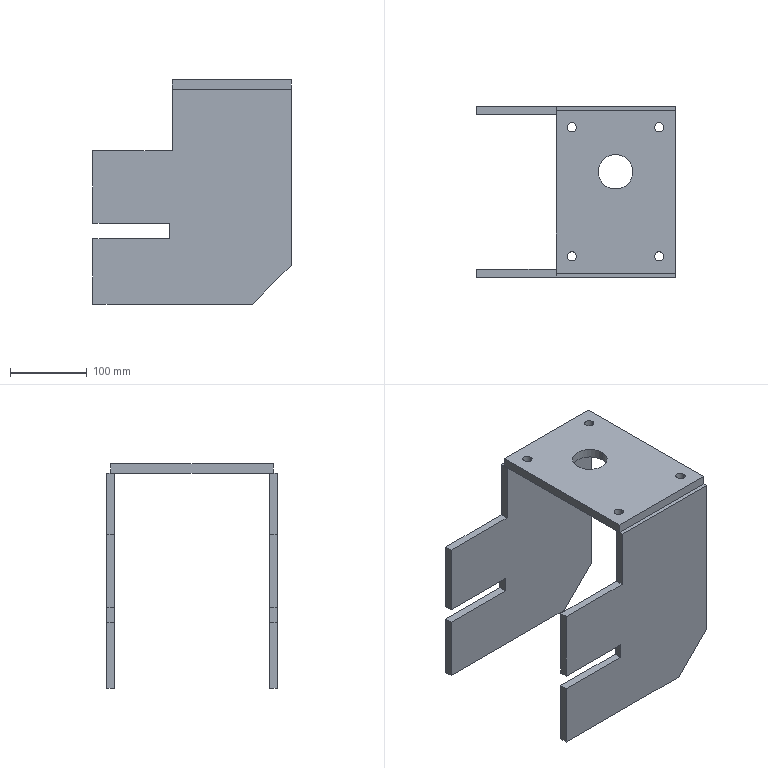Part | SolidWorks | features ICE 2, Chamfer 1, Cut 1, Extrusion 1, HoleWzd 1, MirrorSolid 1 | 3 solids | 42 faces | box 258 x 222 x 292 mm | volume 1584806 mm3 | plane 32 | cylinder 10 | commonest cylinder face diameters 12 x8 45 x2
STEP:
#1=CARTESIAN_POINT('',(22.5,26.,12.));
#2=VERTEX_POINT('',#1);
#3=CARTESIAN_POINT('',(-22.5,26.,12.));
#4=VERTEX_POINT('',#3);
#5=CARTESIAN_POINT('',(0.,26.,12.));
#6=DIRECTION('',(0.,0.,-1.));
#7=DIRECTION('',(1.,0.,0.));
#8=AXIS2_PLACEMENT_3D('',#5,#6,#7);
#9=CIRCLE('',#8,22.5);
#10=EDGE_CURVE('',#2,#4,#9,.T.);
#11=ORIENTED_EDGE('',*,*,#10,.F.);
#12=CARTESIAN_POINT('',(22.5,26.,0.));
#13=VERTEX_POINT('',#12);
#14=CARTESIAN_POINT('',(22.5,26.,12.001));
#15=DIRECTION('',(0.,0.,-1.));
#16=VECTOR('',#15,1000.);
#17=LINE('',#14,#16);
#18=EDGE_CURVE('',#2,#13,#17,.T.);
#19=ORIENTED_EDGE('',*,*,#18,.T.);
#20=CARTESIAN_POINT('',(-22.5,26.,0.));
#21=VERTEX_POINT('',#20);
#22=CARTESIAN_POINT('',(0.,26.,0.));
#23=DIRECTION('',(0.,0.,-1.));
#24=DIRECTION('',(-1.,0.,0.));
#25=AXIS2_PLACEMENT_3D('',#22,#23,#24);
#26=CIRCLE('',#25,22.5);
#27=EDGE_CURVE('',#13,#21,#26,.T.);
#28=ORIENTED_EDGE('',*,*,#27,.T.);
#29=CARTESIAN_POINT('',(-22.5,26.,12.001));
#30=DIRECTION('',(0.,0.,-1.));
#31=VECTOR('',#30,1000.);
#32=LINE('',#29,#31);
#33=EDGE_CURVE('',#4,#21,#32,.T.);
#34=ORIENTED_EDGE('',*,*,#33,.F.);
#35=EDGE_LOOP('',(#11,#19,#28,#34));
#36=FACE_OUTER_BOUND('',#35,.T.);
#37=CARTESIAN_POINT('',(0.,26.,12.001));
#38=DIRECTION('',(0.,0.,-1.));
#39=DIRECTION('',(-1.,0.,0.));
#40=AXIS2_PLACEMENT_3D('',#37,#38,#39);
#41=CYLINDRICAL_SURFACE('',#40,22.5);
#42=ADVANCED_FACE('',(#36),#41,.F.);
#43=CARTESIAN_POINT('',(51.,84.,12.));
#44=VERTEX_POINT('',#43);
#45=CARTESIAN_POINT('',(63.,84.,12.));
#46=VERTEX_POINT('',#45);
#47=CARTESIAN_POINT('',(57.,84.,12.));
#48=DIRECTION('',(0.,0.,1.));
#49=DIRECTION('',(1.,0.,0.));
#50=AXIS2_PLACEMENT_3D('',#47,#48,#49);
#51=CIRCLE('',#50,6.);
#52=EDGE_CURVE('',#44,#46,#51,.T.);
#53=ORIENTED_EDGE('',*,*,#52,.T.);
#54=CARTESIAN_POINT('',(63.,84.,0.));
#55=VERTEX_POINT('',#54);
#56=CARTESIAN_POINT('',(63.,84.,0.));
#57=DIRECTION('',(0.,0.,-1.));
#58=VECTOR('',#57,1000.);
#59=LINE('',#56,#58);
#60=EDGE_CURVE('',#46,#55,#59,.T.);
#61=ORIENTED_EDGE('',*,*,#60,.T.);
#62=CARTESIAN_POINT('',(51.,84.,0.));
#63=VERTEX_POINT('',#62);
#64=CARTESIAN_POINT('',(57.,84.,0.));
#65=DIRECTION('',(0.,0.,-1.));
#66=DIRECTION('',(-1.,0.,0.));
#67=AXIS2_PLACEMENT_3D('',#64,#65,#66);
#68=CIRCLE('',#67,6.);
#69=EDGE_CURVE('',#55,#63,#68,.T.);
#70=ORIENTED_EDGE('',*,*,#69,.T.);
#71=CARTESIAN_POINT('',(51.,84.,0.));
#72=DIRECTION('',(0.,0.,-1.));
#73=VECTOR('',#72,1000.);
#74=LINE('',#71,#73);
#75=EDGE_CURVE('',#44,#63,#74,.T.);
#76=ORIENTED_EDGE('',*,*,#75,.F.);
#77=EDGE_LOOP('',(#53,#61,#70,#76));
#78=FACE_OUTER_BOUND('',#77,.T.);
#79=CARTESIAN_POINT('',(57.,84.,0.));
#80=DIRECTION('',(0.,0.,-1.));
#81=DIRECTION('',(-1.,0.,0.));
#82=AXIS2_PLACEMENT_3D('',#79,#80,#81);
#83=CYLINDRICAL_SURFACE('',#82,6.);
#84=ADVANCED_FACE('',(#78),#83,.F.);
#85=CARTESIAN_POINT('',(-63.,84.,12.));
#86=VERTEX_POINT('',#85);
#87=CARTESIAN_POINT('',(-51.,84.,12.));
#88=VERTEX_POINT('',#87);
#89=CARTESIAN_POINT('',(-57.,84.,12.));
#90=DIRECTION('',(0.,0.,1.));
#91=DIRECTION('',(1.,0.,0.));
#92=AXIS2_PLACEMENT_3D('',#89,#90,#91);
#93=CIRCLE('',#92,6.);
#94=EDGE_CURVE('',#86,#88,#93,.T.);
#95=ORIENTED_EDGE('',*,*,#94,.T.);
#96=CARTESIAN_POINT('',(-51.,84.,0.));
#97=VERTEX_POINT('',#96);
#98=CARTESIAN_POINT('',(-51.,84.,0.));
#99=DIRECTION('',(0.,0.,-1.));
#100=VECTOR('',#99,1000.);
#101=LINE('',#98,#100);
#102=EDGE_CURVE('',#88,#97,#101,.T.);
#103=ORIENTED_EDGE('',*,*,#102,.T.);
#104=CARTESIAN_POINT('',(-63.,84.,0.));
#105=VERTEX_POINT('',#104);
#106=CARTESIAN_POINT('',(-57.,84.,0.));
#107=DIRECTION('',(0.,0.,-1.));
#108=DIRECTION('',(-1.,0.,0.));
#109=AXIS2_PLACEMENT_3D('',#106,#107,#108);
#110=CIRCLE('',#109,6.);
#111=EDGE_CURVE('',#97,#105,#110,.T.);
#112=ORIENTED_EDGE('',*,*,#111,.T.);
#113=CARTESIAN_POINT('',(-63.,84.,0.));
#114=DIRECTION('',(0.,0.,-1.));
#115=VECTOR('',#114,1000.);
#116=LINE('',#113,#115);
#117=EDGE_CURVE('',#86,#105,#116,.T.);
#118=ORIENTED_EDGE('',*,*,#117,.F.);
#119=EDGE_LOOP('',(#95,#103,#112,#118));
#120=FACE_OUTER_BOUND('',#119,.T.);
#121=CARTESIAN_POINT('',(-57.,84.,0.));
#122=DIRECTION('',(0.,0.,-1.));
#123=DIRECTION('',(-1.,0.,0.));
#124=AXIS2_PLACEMENT_3D('',#121,#122,#123);
#125=CYLINDRICAL_SURFACE('',#124,6.);
#126=ADVANCED_FACE('',(#120),#125,.F.);
#127=CARTESIAN_POINT('',(51.,-84.,12.));
#128=VERTEX_POINT('',#127);
#129=CARTESIAN_POINT('',(63.,-84.,12.));
#130=VERTEX_POINT('',#129);
#131=CARTESIAN_POINT('',(57.,-84.,12.));
#132=DIRECTION('',(0.,0.,1.));
#133=DIRECTION('',(1.,0.,0.));
#134=AXIS2_PLACEMENT_3D('',#131,#132,#133);
#135=CIRCLE('',#134,6.);
#136=EDGE_CURVE('',#128,#130,#135,.T.);
#137=ORIENTED_EDGE('',*,*,#136,.T.);
#138=CARTESIAN_POINT('',(63.,-84.,0.));
#139=VERTEX_POINT('',#138);
#140=CARTESIAN_POINT('',(63.,-84.,0.));
#141=DIRECTION('',(0.,0.,-1.));
#142=VECTOR('',#141,1000.);
#143=LINE('',#140,#142);
#144=EDGE_CURVE('',#130,#139,#143,.T.);
#145=ORIENTED_EDGE('',*,*,#144,.T.);
#146=CARTESIAN_POINT('',(51.,-84.,0.));
#147=VERTEX_POINT('',#146);
#148=CARTESIAN_POINT('',(57.,-84.,0.));
#149=DIRECTION('',(0.,0.,-1.));
#150=DIRECTION('',(-1.,0.,0.));
#151=AXIS2_PLACEMENT_3D('',#148,#149,#150);
#152=CIRCLE('',#151,6.);
#153=EDGE_CURVE('',#139,#147,#152,.T.);
#154=ORIENTED_EDGE('',*,*,#153,.T.);
#155=CARTESIAN_POINT('',(51.,-84.,0.));
#156=DIRECTION('',(0.,0.,-1.));
#157=VECTOR('',#156,1000.);
#158=LINE('',#155,#157);
#159=EDGE_CURVE('',#128,#147,#158,.T.);
#160=ORIENTED_EDGE('',*,*,#159,.F.);
#161=EDGE_LOOP('',(#137,#145,#154,#160));
#162=FACE_OUTER_BOUND('',#161,.T.);
#163=CARTESIAN_POINT('',(57.,-84.,0.));
#164=DIRECTION('',(0.,0.,-1.));
#165=DIRECTION('',(-1.,0.,0.));
#166=AXIS2_PLACEMENT_3D('',#163,#164,#165);
#167=CYLINDRICAL_SURFACE('',#166,6.);
#168=ADVANCED_FACE('',(#162),#167,.F.);
#169=CARTESIAN_POINT('',(-63.,-84.,12.));
#170=VERTEX_POINT('',#169);
#171=CARTESIAN_POINT('',(-51.,-84.,12.));
#172=VERTEX_POINT('',#171);
#173=CARTESIAN_POINT('',(-57.,-84.,12.));
#174=DIRECTION('',(0.,0.,1.));
#175=DIRECTION('',(1.,0.,0.));
#176=AXIS2_PLACEMENT_3D('',#173,#174,#175);
#177=CIRCLE('',#176,6.);
#178=EDGE_CURVE('',#170,#172,#177,.T.);
#179=ORIENTED_EDGE('',*,*,#178,.T.);
#180=CARTESIAN_POINT('',(-51.,-84.,0.));
#181=VERTEX_POINT('',#180);
#182=CARTESIAN_POINT('',(-51.,-84.,0.));
#183=DIRECTION('',(0.,0.,-1.));
#184=VECTOR('',#183,1000.);
#185=LINE('',#182,#184);
#186=EDGE_CURVE('',#172,#181,#185,.T.);
#187=ORIENTED_EDGE('',*,*,#186,.T.);
#188=CARTESIAN_POINT('',(-63.,-84.,0.));
#189=VERTEX_POINT('',#188);
#190=CARTESIAN_POINT('',(-57.,-84.,0.));
#191=DIRECTION('',(0.,0.,-1.));
#192=DIRECTION('',(-1.,0.,0.));
#193=AXIS2_PLACEMENT_3D('',#190,#191,#192);
#194=CIRCLE('',#193,6.);
#195=EDGE_CURVE('',#181,#189,#194,.T.);
#196=ORIENTED_EDGE('',*,*,#195,.T.);
#197=CARTESIAN_POINT('',(-63.,-84.,0.));
#198=DIRECTION('',(0.,0.,-1.));
#199=VECTOR('',#198,1000.);
#200=LINE('',#197,#199);
#201=EDGE_CURVE('',#170,#189,#200,.T.);
#202=ORIENTED_EDGE('',*,*,#201,.F.);
#203=EDGE_LOOP('',(#179,#187,#196,#202));
#204=FACE_OUTER_BOUND('',#203,.T.);
#205=CARTESIAN_POINT('',(-57.,-84.,0.));
#206=DIRECTION('',(0.,0.,-1.));
#207=DIRECTION('',(-1.,0.,0.));
#208=AXIS2_PLACEMENT_3D('',#205,#206,#207);
#209=CYLINDRICAL_SURFACE('',#208,6.);
#210=ADVANCED_FACE('',(#204),#209,.F.);
#211=CARTESIAN_POINT('',(0.,26.,0.));
#212=DIRECTION('',(0.,0.,-1.));
#213=DIRECTION('',(-1.,0.,0.));
#214=AXIS2_PLACEMENT_3D('',#211,#212,#213);
#215=CIRCLE('',#214,22.5);
#216=EDGE_CURVE('',#21,#13,#215,.T.);
#217=ORIENTED_EDGE('',*,*,#216,.F.);
#218=ORIENTED_EDGE('',*,*,#27,.F.);
#219=EDGE_LOOP('',(#217,#218));
#220=FACE_BOUND('',#219,.T.);
#221=CARTESIAN_POINT('',(57.,84.,0.));
#222=DIRECTION('',(0.,0.,-1.));
#223=DIRECTION('',(-1.,0.,0.));
#224=AXIS2_PLACEMENT_3D('',#221,#222,#223);
#225=CIRCLE('',#224,6.);
#226=EDGE_CURVE('',#63,#55,#225,.T.);
#227=ORIENTED_EDGE('',*,*,#226,.F.);
#228=ORIENTED_EDGE('',*,*,#69,.F.);
#229=EDGE_LOOP('',(#227,#228));
#230=FACE_BOUND('',#229,.T.);
#231=CARTESIAN_POINT('',(-57.,84.,0.));
#232=DIRECTION('',(0.,0.,-1.));
#233=DIRECTION('',(-1.,0.,0.));
#234=AXIS2_PLACEMENT_3D('',#231,#232,#233);
#235=CIRCLE('',#234,6.);
#236=EDGE_CURVE('',#105,#97,#235,.T.);
#237=ORIENTED_EDGE('',*,*,#236,.F.);
#238=ORIENTED_EDGE('',*,*,#111,.F.);
#239=EDGE_LOOP('',(#237,#238));
#240=FACE_BOUND('',#239,.T.);
#241=CARTESIAN_POINT('',(57.,-84.,0.));
#242=DIRECTION('',(0.,0.,-1.));
#243=DIRECTION('',(-1.,0.,0.));
#244=AXIS2_PLACEMENT_3D('',#241,#242,#243);
#245=CIRCLE('',#244,6.);
#246=EDGE_CURVE('',#147,#139,#245,.T.);
#247=ORIENTED_EDGE('',*,*,#246,.F.);
#248=ORIENTED_EDGE('',*,*,#153,.F.);
#249=EDGE_LOOP('',(#247,#248));
#250=FACE_BOUND('',#249,.T.);
#251=CARTESIAN_POINT('',(-77.5,106.,0.));
#252=VERTEX_POINT('',#251);
#253=CARTESIAN_POINT('',(-77.5,-106.,0.));
#254=VERTEX_POINT('',#253);
#255=CARTESIAN_POINT('',(-77.5,-106.,0.));
#256=DIRECTION('',(0.,-1.,0.));
#257=VECTOR('',#256,1000.);
#258=LINE('',#255,#257);
#259=EDGE_CURVE('',#252,#254,#258,.T.);
#260=ORIENTED_EDGE('',*,*,#259,.F.);
#261=CARTESIAN_POINT('',(77.5,106.,0.));
#262=VERTEX_POINT('',#261);
#263=CARTESIAN_POINT('',(77.5,106.,0.));
#264=DIRECTION('',(-1.,0.,0.));
#265=VECTOR('',#264,1000.);
#266=LINE('',#263,#265);
#267=EDGE_CURVE('',#262,#252,#266,.T.);
#268=ORIENTED_EDGE('',*,*,#267,.F.);
#269=CARTESIAN_POINT('',(77.5,-106.,0.));
#270=VERTEX_POINT('',#269);
#271=CARTESIAN_POINT('',(77.5,-106.,0.));
#272=DIRECTION('',(0.,1.,0.));
#273=VECTOR('',#272,1000.);
#274=LINE('',#271,#273);
#275=EDGE_CURVE('',#270,#262,#274,.T.);
#276=ORIENTED_EDGE('',*,*,#275,.F.);
#277=CARTESIAN_POINT('',(77.5,-106.,0.));
#278=DIRECTION('',(1.,0.,0.));
#279=VECTOR('',#278,1000.);
#280=LINE('',#277,#279);
#281=EDGE_CURVE('',#254,#270,#280,.T.);
#282=ORIENTED_EDGE('',*,*,#281,.F.);
#283=EDGE_LOOP('',(#260,#268,#276,#282));
#284=FACE_OUTER_BOUND('',#283,.T.);
#285=CARTESIAN_POINT('',(-57.,-84.,0.));
#286=DIRECTION('',(0.,0.,-1.));
#287=DIRECTION('',(-1.,0.,0.));
#288=AXIS2_PLACEMENT_3D('',#285,#286,#287);
#289=CIRCLE('',#288,6.);
#290=EDGE_CURVE('',#189,#181,#289,.T.);
#291=ORIENTED_EDGE('',*,*,#290,.F.);
#292=ORIENTED_EDGE('',*,*,#195,.F.);
#293=EDGE_LOOP('',(#291,#292));
#294=FACE_BOUND('',#293,.T.);
#295=CARTESIAN_POINT('',(0.,0.,0.));
#296=DIRECTION('',(0.,0.,1.));
#297=DIRECTION('',(1.,0.,0.));
#298=AXIS2_PLACEMENT_3D('',#295,#296,#297);
#299=PLANE('',#298);
#300=ADVANCED_FACE('',(#220,#230,#240,#250,#284,#294),#299,.F.);
#301=ORIENTED_EDGE('',*,*,#259,.T.);
#302=CARTESIAN_POINT('',(-77.5,-106.,12.));
#303=VERTEX_POINT('',#302);
#304=CARTESIAN_POINT('',(-77.5,-106.,12.));
#305=DIRECTION('',(0.,0.,-1.));
#306=VECTOR('',#305,1000.);
#307=LINE('',#304,#306);
#308=EDGE_CURVE('',#303,#254,#307,.T.);
#309=ORIENTED_EDGE('',*,*,#308,.F.);
#310=CARTESIAN_POINT('',(-77.5,106.,12.));
#311=VERTEX_POINT('',#310);
#312=CARTESIAN_POINT('',(-77.5,-106.,12.));
#313=DIRECTION('',(0.,-1.,0.));
#314=VECTOR('',#313,1000.);
#315=LINE('',#312,#314);
#316=EDGE_CURVE('',#311,#303,#315,.T.);
#317=ORIENTED_EDGE('',*,*,#316,.F.);
#318=CARTESIAN_POINT('',(-77.5,106.,12.));
#319=DIRECTION('',(0.,0.,-1.));
#320=VECTOR('',#319,1000.);
#321=LINE('',#318,#320);
#322=EDGE_CURVE('',#311,#252,#321,.T.);
#323=ORIENTED_EDGE('',*,*,#322,.T.);
#324=EDGE_LOOP('',(#301,#309,#317,#323));
#325=FACE_OUTER_BOUND('',#324,.T.);
#326=CARTESIAN_POINT('',(-77.5,-106.,12.));
#327=DIRECTION('',(1.,0.,0.));
#328=DIRECTION('',(0.,0.,-1.));
#329=AXIS2_PLACEMENT_3D('',#326,#327,#328);
#330=PLANE('',#329);
#331=ADVANCED_FACE('',(#325),#330,.F.);
#332=ORIENTED_EDGE('',*,*,#281,.T.);
#333=CARTESIAN_POINT('',(77.5,-106.,12.));
#334=VERTEX_POINT('',#333);
#335=CARTESIAN_POINT('',(77.5,-106.,12.));
#336=DIRECTION('',(0.,0.,-1.));
#337=VECTOR('',#336,1000.);
#338=LINE('',#335,#337);
#339=EDGE_CURVE('',#334,#270,#338,.T.);
#340=ORIENTED_EDGE('',*,*,#339,.F.);
#341=CARTESIAN_POINT('',(77.5,-106.,12.));
#342=DIRECTION('',(1.,0.,0.));
#343=VECTOR('',#342,1000.);
#344=LINE('',#341,#343);
#345=EDGE_CURVE('',#303,#334,#344,.T.);
#346=ORIENTED_EDGE('',*,*,#345,.F.);
#347=ORIENTED_EDGE('',*,*,#308,.T.);
#348=EDGE_LOOP('',(#332,#340,#346,#347));
#349=FACE_OUTER_BOUND('',#348,.T.);
#350=CARTESIAN_POINT('',(77.5,-106.,12.));
#351=DIRECTION('',(0.,1.,0.));
#352=DIRECTION('',(0.,0.,1.));
#353=AXIS2_PLACEMENT_3D('',#350,#351,#352);
#354=PLANE('',#353);
#355=ADVANCED_FACE('',(#349),#354,.F.);
#356=ORIENTED_EDGE('',*,*,#275,.T.);
#357=CARTESIAN_POINT('',(77.5,106.,12.));
#358=VERTEX_POINT('',#357);
#359=CARTESIAN_POINT('',(77.5,106.,12.));
#360=DIRECTION('',(0.,0.,-1.));
#361=VECTOR('',#360,1000.);
#362=LINE('',#359,#361);
#363=EDGE_CURVE('',#358,#262,#362,.T.);
#364=ORIENTED_EDGE('',*,*,#363,.F.);
#365=CARTESIAN_POINT('',(77.5,-106.,12.));
#366=DIRECTION('',(0.,1.,0.));
#367=VECTOR('',#366,1000.);
#368=LINE('',#365,#367);
#369=EDGE_CURVE('',#334,#358,#368,.T.);
#370=ORIENTED_EDGE('',*,*,#369,.F.);
#371=ORIENTED_EDGE('',*,*,#339,.T.);
#372=EDGE_LOOP('',(#356,#364,#370,#371));
#373=FACE_OUTER_BOUND('',#372,.T.);
#374=CARTESIAN_POINT('',(77.5,-106.,12.));
#375=DIRECTION('',(-1.,0.,0.));
#376=DIRECTION('',(0.,0.,1.));
#377=AXIS2_PLACEMENT_3D('',#374,#375,#376);
#378=PLANE('',#377);
#379=ADVANCED_FACE('',(#373),#378,.F.);
#380=ORIENTED_EDGE('',*,*,#267,.T.);
#381=ORIENTED_EDGE('',*,*,#322,.F.);
#382=CARTESIAN_POINT('',(77.5,106.,12.));
#383=DIRECTION('',(-1.,0.,0.));
#384=VECTOR('',#383,1000.);
#385=LINE('',#382,#384);
#386=EDGE_CURVE('',#358,#311,#385,.T.);
#387=ORIENTED_EDGE('',*,*,#386,.F.);
#388=ORIENTED_EDGE('',*,*,#363,.T.);
#389=EDGE_LOOP('',(#380,#381,#387,#388));
#390=FACE_OUTER_BOUND('',#389,.T.);
#391=CARTESIAN_POINT('',(77.5,106.,12.));
#392=DIRECTION('',(0.,-1.,0.));
#393=DIRECTION('',(0.,0.,-1.));
#394=AXIS2_PLACEMENT_3D('',#391,#392,#393);
#395=PLANE('',#394);
#396=ADVANCED_FACE('',(#390),#395,.F.);
#397=CARTESIAN_POINT('',(0.,26.,12.));
#398=DIRECTION('',(0.,0.,-1.));
#399=DIRECTION('',(1.,0.,0.));
#400=AXIS2_PLACEMENT_3D('',#397,#398,#399);
#401=CIRCLE('',#400,22.5);
#402=EDGE_CURVE('',#4,#2,#401,.T.);
#403=ORIENTED_EDGE('',*,*,#402,.T.);
#404=ORIENTED_EDGE('',*,*,#10,.T.);
#405=EDGE_LOOP('',(#403,#404));
#406=FACE_BOUND('',#405,.T.);
#407=ORIENTED_EDGE('',*,*,#52,.F.);
#408=CARTESIAN_POINT('',(57.,84.,12.));
#409=DIRECTION('',(0.,0.,1.));
#410=DIRECTION('',(1.,0.,0.));
#411=AXIS2_PLACEMENT_3D('',#408,#409,#410);
#412=CIRCLE('',#411,6.);
#413=EDGE_CURVE('',#46,#44,#412,.T.);
#414=ORIENTED_EDGE('',*,*,#413,.F.);
#415=EDGE_LOOP('',(#407,#414));
#416=FACE_BOUND('',#415,.T.);
#417=ORIENTED_EDGE('',*,*,#94,.F.);
#418=CARTESIAN_POINT('',(-57.,84.,12.));
#419=DIRECTION('',(0.,0.,1.));
#420=DIRECTION('',(1.,0.,0.));
#421=AXIS2_PLACEMENT_3D('',#418,#419,#420);
#422=CIRCLE('',#421,6.);
#423=EDGE_CURVE('',#88,#86,#422,.T.);
#424=ORIENTED_EDGE('',*,*,#423,.F.);
#425=EDGE_LOOP('',(#417,#424));
#426=FACE_BOUND('',#425,.T.);
#427=ORIENTED_EDGE('',*,*,#136,.F.);
#428=CARTESIAN_POINT('',(57.,-84.,12.));
#429=DIRECTION('',(0.,0.,1.));
#430=DIRECTION('',(1.,0.,0.));
#431=AXIS2_PLACEMENT_3D('',#428,#429,#430);
#432=CIRCLE('',#431,6.);
#433=EDGE_CURVE('',#130,#128,#432,.T.);
#434=ORIENTED_EDGE('',*,*,#433,.F.);
#435=EDGE_LOOP('',(#427,#434));
#436=FACE_BOUND('',#435,.T.);
#437=ORIENTED_EDGE('',*,*,#178,.F.);
#438=CARTESIAN_POINT('',(-57.,-84.,12.));
#439=DIRECTION('',(0.,0.,1.));
#440=DIRECTION('',(1.,0.,0.));
#441=AXIS2_PLACEMENT_3D('',#438,#439,#440);
#442=CIRCLE('',#441,6.);
#443=EDGE_CURVE('',#172,#170,#442,.T.);
#444=ORIENTED_EDGE('',*,*,#443,.F.);
#445=EDGE_LOOP('',(#437,#444));
#446=FACE_BOUND('',#445,.T.);
#447=ORIENTED_EDGE('',*,*,#316,.T.);
#448=ORIENTED_EDGE('',*,*,#345,.T.);
#449=ORIENTED_EDGE('',*,*,#369,.T.);
#450=ORIENTED_EDGE('',*,*,#386,.T.);
#451=EDGE_LOOP('',(#447,#448,#449,#450));
#452=FACE_OUTER_BOUND('',#451,.T.);
#453=CARTESIAN_POINT('',(0.,0.,12.));
#454=DIRECTION('',(0.,0.,1.));
#455=DIRECTION('',(1.,0.,0.));
#456=AXIS2_PLACEMENT_3D('',#453,#454,#455);
#457=PLANE('',#456);
#458=ADVANCED_FACE('',(#406,#416,#426,#436,#446,#452),#457,.T.);
#459=ORIENTED_EDGE('',*,*,#186,.F.);
#460=ORIENTED_EDGE('',*,*,#443,.T.);
#461=ORIENTED_EDGE('',*,*,#201,.T.);
#462=ORIENTED_EDGE('',*,*,#290,.T.);
#463=EDGE_LOOP('',(#459,#460,#461,#462));
#464=FACE_OUTER_BOUND('',#463,.T.);
#465=CARTESIAN_POINT('',(-57.,-84.,0.));
#466=DIRECTION('',(0.,0.,-1.));
#467=DIRECTION('',(-1.,0.,0.));
#468=AXIS2_PLACEMENT_3D('',#465,#466,#467);
#469=CYLINDRICAL_SURFACE('',#468,6.);
#470=ADVANCED_FACE('',(#464),#469,.F.);
#471=ORIENTED_EDGE('',*,*,#144,.F.);
#472=ORIENTED_EDGE('',*,*,#433,.T.);
#473=ORIENTED_EDGE('',*,*,#159,.T.);
#474=ORIENTED_EDGE('',*,*,#246,.T.);
#475=EDGE_LOOP('',(#471,#472,#473,#474));
#476=FACE_OUTER_BOUND('',#475,.T.);
#477=CARTESIAN_POINT('',(57.,-84.,0.));
#478=DIRECTION('',(0.,0.,-1.));
#479=DIRECTION('',(-1.,0.,0.));
#480=AXIS2_PLACEMENT_3D('',#477,#478,#479);
#481=CYLINDRICAL_SURFACE('',#480,6.);
#482=ADVANCED_FACE('',(#476),#481,.F.);
#483=ORIENTED_EDGE('',*,*,#102,.F.);
#484=ORIENTED_EDGE('',*,*,#423,.T.);
#485=ORIENTED_EDGE('',*,*,#117,.T.);
#486=ORIENTED_EDGE('',*,*,#236,.T.);
#487=EDGE_LOOP('',(#483,#484,#485,#486));
#488=FACE_OUTER_BOUND('',#487,.T.);
#489=CARTESIAN_POINT('',(-57.,84.,0.));
#490=DIRECTION('',(0.,0.,-1.));
#491=DIRECTION('',(-1.,0.,0.));
#492=AXIS2_PLACEMENT_3D('',#489,#490,#491);
#493=CYLINDRICAL_SURFACE('',#492,6.);
#494=ADVANCED_FACE('',(#488),#493,.F.);
#495=ORIENTED_EDGE('',*,*,#60,.F.);
#496=ORIENTED_EDGE('',*,*,#413,.T.);
#497=ORIENTED_EDGE('',*,*,#75,.T.);
#498=ORIENTED_EDGE('',*,*,#226,.T.);
#499=EDGE_LOOP('',(#495,#496,#497,#498));
#500=FACE_OUTER_BOUND('',#499,.T.);
#501=CARTESIAN_POINT('',(57.,84.,0.));
#502=DIRECTION('',(0.,0.,-1.));
#503=DIRECTION('',(-1.,0.,0.));
#504=AXIS2_PLACEMENT_3D('',#501,#502,#503);
#505=CYLINDRICAL_SURFACE('',#504,6.);
#506=ADVANCED_FACE('',(#500),#505,.F.);
#507=ORIENTED_EDGE('',*,*,#18,.F.);
#508=ORIENTED_EDGE('',*,*,#402,.F.);
#509=ORIENTED_EDGE('',*,*,#33,.T.);
#510=ORIENTED_EDGE('',*,*,#216,.T.);
#511=EDGE_LOOP('',(#507,#508,#509,#510));
#512=FACE_OUTER_BOUND('',#511,.T.);
#513=CARTESIAN_POINT('',(0.,26.,12.001));
#514=DIRECTION('',(0.,0.,-1.));
#515=DIRECTION('',(-1.,0.,0.));
#516=AXIS2_PLACEMENT_3D('',#513,#514,#515);
#517=CYLINDRICAL_SURFACE('',#516,22.5);
#518=ADVANCED_FACE('',(#512),#517,.F.);
#519=CLOSED_SHELL('',(#42,#84,#126,#168,#210,#300,#331,#355,#379,#396,#458,#470,#482,#494,#506,#518));
#520=MANIFOLD_SOLID_BREP('',#519);
#521=CARTESIAN_POINT('',(-180.5,101.,-280.));
#522=VERTEX_POINT('',#521);
#523=CARTESIAN_POINT('',(-180.5,101.,-195.));
#524=VERTEX_POINT('',#523);
#525=CARTESIAN_POINT('',(-180.5,101.,-280.));
#526=DIRECTION('',(0.,0.,1.));
#527=VECTOR('',#526,1000.);
#528=LINE('',#525,#527);
#529=EDGE_CURVE('',#522,#524,#528,.T.);
#530=ORIENTED_EDGE('',*,*,#529,.T.);
#531=CARTESIAN_POINT('',(-180.5,111.,-195.));
#532=VERTEX_POINT('',#531);
#533=CARTESIAN_POINT('',(-180.5,-111.,-195.));
#534=DIRECTION('',(0.,1.,0.));
#535=VECTOR('',#534,1000.);
#536=LINE('',#533,#535);
#537=EDGE_CURVE('',#524,#532,#536,.T.);
#538=ORIENTED_EDGE('',*,*,#537,.T.);
#539=CARTESIAN_POINT('',(-180.5,111.,-280.));
#540=VERTEX_POINT('',#539);
#541=CARTESIAN_POINT('',(-180.5,111.,-280.));
#542=DIRECTION('',(0.,0.,1.));
#543=VECTOR('',#542,1000.);
#544=LINE('',#541,#543);
#545=EDGE_CURVE('',#540,#532,#544,.T.);
#546=ORIENTED_EDGE('',*,*,#545,.F.);
#547=CARTESIAN_POINT('',(-180.5,111.,-280.));
#548=DIRECTION('',(0.,-1.,0.));
#549=VECTOR('',#548,1000.);
#550=LINE('',#547,#549);
#551=EDGE_CURVE('',#540,#522,#550,.T.);
#552=ORIENTED_EDGE('',*,*,#551,.T.);
#553=EDGE_LOOP('',(#530,#538,#546,#552));
#554=FACE_OUTER_BOUND('',#553,.T.);
#555=CARTESIAN_POINT('',(-180.5,111.,-280.));
#556=DIRECTION('',(1.,0.,0.));
#557=DIRECTION('',(0.,0.,-1.));
#558=AXIS2_PLACEMENT_3D('',#555,#556,#557);
#559=PLANE('',#558);
#560=ADVANCED_FACE('',(#554),#559,.F.);
#561=CARTESIAN_POINT('',(77.5,101.,0.));
#562=VERTEX_POINT('',#561);
#563=CARTESIAN_POINT('',(77.5,101.,-230.));
#564=VERTEX_POINT('',#563);
#565=CARTESIAN_POINT('',(77.5,101.,0.));
#566=DIRECTION('',(0.,0.,-1.));
#567=VECTOR('',#566,1000.);
#568=LINE('',#565,#567);
#569=EDGE_CURVE('',#562,#564,#568,.T.);
#570=ORIENTED_EDGE('',*,*,#569,.T.);
#571=CARTESIAN_POINT('',(77.5,111.,-230.));
#572=VERTEX_POINT('',#571);
#573=CARTESIAN_POINT('',(77.5,111.,-230.));
#574=DIRECTION('',(0.,1.,0.));
#575=VECTOR('',#574,1000.);
#576=LINE('',#573,#575);
#577=EDGE_CURVE('',#564,#572,#576,.T.);
#578=ORIENTED_EDGE('',*,*,#577,.T.);
#579=CARTESIAN_POINT('',(77.5,111.,0.));
#580=VERTEX_POINT('',#579);
#581=CARTESIAN_POINT('',(77.5,111.,0.));
#582=DIRECTION('',(0.,0.,-1.));
#583=VECTOR('',#582,1000.);
#584=LINE('',#581,#583);
#585=EDGE_CURVE('',#580,#572,#584,.T.);
#586=ORIENTED_EDGE('',*,*,#585,.F.);
#587=CARTESIAN_POINT('',(77.5,111.,0.));
#588=DIRECTION('',(0.,-1.,0.));
#589=VECTOR('',#588,1000.);
#590=LINE('',#587,#589);
#591=EDGE_CURVE('',#580,#562,#590,.T.);
#592=ORIENTED_EDGE('',*,*,#591,.T.);
#593=EDGE_LOOP('',(#570,#578,#586,#592));
#594=FACE_OUTER_BOUND('',#593,.T.);
#595=CARTESIAN_POINT('',(77.5,111.,0.));
#596=DIRECTION('',(-1.,0.,0.));
#597=DIRECTION('',(0.,0.,1.));
#598=AXIS2_PLACEMENT_3D('',#595,#596,#597);
#599=PLANE('',#598);
#600=ADVANCED_FACE('',(#594),#599,.F.);
#601=CARTESIAN_POINT('',(27.5,111.,-280.));
#602=VERTEX_POINT('',#601);
#603=CARTESIAN_POINT('',(77.5,111.,-280.));
#604=DIRECTION('',(-1.,0.,0.));
#605=VECTOR('',#604,1000.);
#606=LINE('',#603,#605);
#607=EDGE_CURVE('',#602,#540,#606,.T.);
#608=ORIENTED_EDGE('',*,*,#607,.F.);
#609=CARTESIAN_POINT('',(27.5,101.,-280.));
#610=VERTEX_POINT('',#609);
#611=CARTESIAN_POINT('',(27.5,111.,-280.));
#612=DIRECTION('',(0.,-1.,0.));
#613=VECTOR('',#612,1000.);
#614=LINE('',#611,#613);
#615=EDGE_CURVE('',#602,#610,#614,.T.);
#616=ORIENTED_EDGE('',*,*,#615,.T.);
#617=CARTESIAN_POINT('',(77.5,101.,-280.));
#618=DIRECTION('',(-1.,0.,0.));
#619=VECTOR('',#618,1000.);
#620=LINE('',#617,#619);
#621=EDGE_CURVE('',#610,#522,#620,.T.);
#622=ORIENTED_EDGE('',*,*,#621,.T.);
#623=ORIENTED_EDGE('',*,*,#551,.F.);
#624=EDGE_LOOP('',(#608,#616,#622,#623));
#625=FACE_OUTER_BOUND('',#624,.T.);
#626=CARTESIAN_POINT('',(77.5,111.,-280.));
#627=DIRECTION('',(0.,0.,1.));
#628=DIRECTION('',(1.,0.,0.));
#629=AXIS2_PLACEMENT_3D('',#626,#627,#628);
#630=PLANE('',#629);
#631=ADVANCED_FACE('',(#625),#630,.F.);
#632=CARTESIAN_POINT('',(-180.5,111.,-175.));
#633=VERTEX_POINT('',#632);
#634=CARTESIAN_POINT('',(-180.5,111.,-80.));
#635=VERTEX_POINT('',#634);
#636=CARTESIAN_POINT('',(-180.5,111.,-280.));
#637=DIRECTION('',(0.,0.,1.));
#638=VECTOR('',#637,1000.);
#639=LINE('',#636,#638);
#640=EDGE_CURVE('',#633,#635,#639,.T.);
#641=ORIENTED_EDGE('',*,*,#640,.F.);
#642=CARTESIAN_POINT('',(-180.5,101.,-175.));
#643=VERTEX_POINT('',#642);
#644=CARTESIAN_POINT('',(-180.5,-111.,-175.));
#645=DIRECTION('',(0.,1.,0.));
#646=VECTOR('',#645,1000.);
#647=LINE('',#644,#646);
#648=EDGE_CURVE('',#643,#633,#647,.T.);
#649=ORIENTED_EDGE('',*,*,#648,.F.);
#650=CARTESIAN_POINT('',(-180.5,101.,-80.));
#651=VERTEX_POINT('',#650);
#652=CARTESIAN_POINT('',(-180.5,101.,-280.));
#653=DIRECTION('',(0.,0.,1.));
#654=VECTOR('',#653,1000.);
#655=LINE('',#652,#654);
#656=EDGE_CURVE('',#643,#651,#655,.T.);
#657=ORIENTED_EDGE('',*,*,#656,.T.);
#658=CARTESIAN_POINT('',(-180.5,111.,-80.));
#659=DIRECTION('',(0.,-1.,0.));
#660=VECTOR('',#659,1000.);
#661=LINE('',#658,#660);
#662=EDGE_CURVE('',#635,#651,#661,.T.);
#663=ORIENTED_EDGE('',*,*,#662,.F.);
#664=EDGE_LOOP('',(#641,#649,#657,#663));
#665=FACE_OUTER_BOUND('',#664,.T.);
#666=CARTESIAN_POINT('',(-180.5,111.,-280.));
#667=DIRECTION('',(1.,0.,0.));
#668=DIRECTION('',(0.,0.,-1.));
#669=AXIS2_PLACEMENT_3D('',#666,#667,#668);
#670=PLANE('',#669);
#671=ADVANCED_FACE('',(#665),#670,.F.);
#672=CARTESIAN_POINT('',(-77.5,101.,-80.));
#673=VERTEX_POINT('',#672);
#674=CARTESIAN_POINT('',(-77.5,101.,-80.));
#675=DIRECTION('',(1.,0.,0.));
#676=VECTOR('',#675,1000.);
#677=LINE('',#674,#676);
#678=EDGE_CURVE('',#651,#673,#677,.T.);
#679=ORIENTED_EDGE('',*,*,#678,.T.);
#680=CARTESIAN_POINT('',(-77.5,111.,-80.));
#681=VERTEX_POINT('',#680);
#682=CARTESIAN_POINT('',(-77.5,111.,-80.));
#683=DIRECTION('',(0.,-1.,0.));
#684=VECTOR('',#683,1000.);
#685=LINE('',#682,#684);
#686=EDGE_CURVE('',#681,#673,#685,.T.);
#687=ORIENTED_EDGE('',*,*,#686,.F.);
#688=CARTESIAN_POINT('',(-77.5,111.,-80.));
#689=DIRECTION('',(1.,0.,0.));
#690=VECTOR('',#689,1000.);
#691=LINE('',#688,#690);
#692=EDGE_CURVE('',#635,#681,#691,.T.);
#693=ORIENTED_EDGE('',*,*,#692,.F.);
#694=ORIENTED_EDGE('',*,*,#662,.T.);
#695=EDGE_LOOP('',(#679,#687,#693,#694));
#696=FACE_OUTER_BOUND('',#695,.T.);
#697=CARTESIAN_POINT('',(-77.5,111.,-80.));
#698=DIRECTION('',(0.,0.,-1.));
#699=DIRECTION('',(-1.,0.,0.));
#700=AXIS2_PLACEMENT_3D('',#697,#698,#699);
#701=PLANE('',#700);
#702=ADVANCED_FACE('',(#696),#701,.F.);
#703=CARTESIAN_POINT('',(-77.5,101.,0.));
#704=VERTEX_POINT('',#703);
#705=CARTESIAN_POINT('',(-77.5,101.,0.));
#706=DIRECTION('',(0.,0.,1.));
#707=VECTOR('',#706,1000.);
#708=LINE('',#705,#707);
#709=EDGE_CURVE('',#673,#704,#708,.T.);
#710=ORIENTED_EDGE('',*,*,#709,.T.);
#711=CARTESIAN_POINT('',(-77.5,111.,0.));
#712=VERTEX_POINT('',#711);
#713=CARTESIAN_POINT('',(-77.5,111.,0.));
#714=DIRECTION('',(0.,-1.,0.));
#715=VECTOR('',#714,1000.);
#716=LINE('',#713,#715);
#717=EDGE_CURVE('',#712,#704,#716,.T.);
#718=ORIENTED_EDGE('',*,*,#717,.F.);
#719=CARTESIAN_POINT('',(-77.5,111.,0.));
#720=DIRECTION('',(0.,0.,1.));
#721=VECTOR('',#720,1000.);
#722=LINE('',#719,#721);
#723=EDGE_CURVE('',#681,#712,#722,.T.);
#724=ORIENTED_EDGE('',*,*,#723,.F.);
#725=ORIENTED_EDGE('',*,*,#686,.T.);
#726=EDGE_LOOP('',(#710,#718,#724,#725));
#727=FACE_OUTER_BOUND('',#726,.T.);
#728=CARTESIAN_POINT('',(-77.5,111.,0.));
#729=DIRECTION('',(1.,0.,0.));
#730=DIRECTION('',(0.,0.,-1.));
#731=AXIS2_PLACEMENT_3D('',#728,#729,#730);
#732=PLANE('',#731);
#733=ADVANCED_FACE('',(#727),#732,.F.);
#734=CARTESIAN_POINT('',(77.5,101.,0.));
#735=DIRECTION('',(1.,0.,0.));
#736=VECTOR('',#735,1000.);
#737=LINE('',#734,#736);
#738=EDGE_CURVE('',#704,#562,#737,.T.);
#739=ORIENTED_EDGE('',*,*,#738,.T.);
#740=ORIENTED_EDGE('',*,*,#591,.F.);
#741=CARTESIAN_POINT('',(77.5,111.,0.));
#742=DIRECTION('',(1.,0.,0.));
#743=VECTOR('',#742,1000.);
#744=LINE('',#741,#743);
#745=EDGE_CURVE('',#712,#580,#744,.T.);
#746=ORIENTED_EDGE('',*,*,#745,.F.);
#747=ORIENTED_EDGE('',*,*,#717,.T.);
#748=EDGE_LOOP('',(#739,#740,#746,#747));
#749=FACE_OUTER_BOUND('',#748,.T.);
#750=CARTESIAN_POINT('',(77.5,111.,0.));
#751=DIRECTION('',(0.,0.,-1.));
#752=DIRECTION('',(-1.,0.,0.));
#753=AXIS2_PLACEMENT_3D('',#750,#751,#752);
#754=PLANE('',#753);
#755=ADVANCED_FACE('',(#749),#754,.F.);
#756=CARTESIAN_POINT('',(-80.5,111.,-195.));
#757=VERTEX_POINT('',#756);
#758=CARTESIAN_POINT('',(-180.5,111.,-195.));
#759=DIRECTION('',(-1.,0.,0.));
#760=VECTOR('',#759,1000.);
#761=LINE('',#758,#760);
#762=EDGE_CURVE('',#757,#532,#761,.T.);
#763=ORIENTED_EDGE('',*,*,#762,.F.);
#764=CARTESIAN_POINT('',(-80.5,111.,-175.));
#765=VERTEX_POINT('',#764);
#766=CARTESIAN_POINT('',(-80.5,111.,-195.));
#767=DIRECTION('',(0.,0.,-1.));
#768=VECTOR('',#767,1000.);
#769=LINE('',#766,#768);
#770=EDGE_CURVE('',#765,#757,#769,.T.);
#771=ORIENTED_EDGE('',*,*,#770,.F.);
#772=CARTESIAN_POINT('',(-180.5,111.,-175.));
#773=DIRECTION('',(1.,0.,0.));
#774=VECTOR('',#773,1000.);
#775=LINE('',#772,#774);
#776=EDGE_CURVE('',#633,#765,#775,.T.);
#777=ORIENTED_EDGE('',*,*,#776,.F.);
#778=ORIENTED_EDGE('',*,*,#640,.T.);
#779=ORIENTED_EDGE('',*,*,#692,.T.);
#780=ORIENTED_EDGE('',*,*,#723,.T.);
#781=ORIENTED_EDGE('',*,*,#745,.T.);
#782=ORIENTED_EDGE('',*,*,#585,.T.);
#783=CARTESIAN_POINT('',(153.75,111.,-153.75));
#784=DIRECTION('',(-0.7071,0.,-0.7071));
#785=VECTOR('',#784,1000.);
#786=LINE('',#783,#785);
#787=EDGE_CURVE('',#572,#602,#786,.T.);
#788=ORIENTED_EDGE('',*,*,#787,.T.);
#789=ORIENTED_EDGE('',*,*,#607,.T.);
#790=ORIENTED_EDGE('',*,*,#545,.T.);
#791=EDGE_LOOP('',(#763,#771,#777,#778,#779,#780,#781,#782,#788,#789,#790));
#792=FACE_OUTER_BOUND('',#791,.T.);
#793=CARTESIAN_POINT('',(0.,111.,0.));
#794=DIRECTION('',(0.,1.,0.));
#795=DIRECTION('',(0.,0.,1.));
#796=AXIS2_PLACEMENT_3D('',#793,#794,#795);
#797=PLANE('',#796);
#798=ADVANCED_FACE('',(#792),#797,.T.);
#799=CARTESIAN_POINT('',(-80.5,101.,-175.));
#800=VERTEX_POINT('',#799);
#801=CARTESIAN_POINT('',(-80.5,101.,-195.));
#802=VERTEX_POINT('',#801);
#803=CARTESIAN_POINT('',(-80.5,101.,0.));
#804=DIRECTION('',(0.,0.,-1.));
#805=VECTOR('',#804,1000.);
#806=LINE('',#803,#805);
#807=EDGE_CURVE('',#800,#802,#806,.T.);
#808=ORIENTED_EDGE('',*,*,#807,.T.);
#809=CARTESIAN_POINT('',(0.,101.,-195.));
#810=DIRECTION('',(-1.,0.,0.));
#811=VECTOR('',#810,1000.);
#812=LINE('',#809,#811);
#813=EDGE_CURVE('',#802,#524,#812,.T.);
#814=ORIENTED_EDGE('',*,*,#813,.T.);
#815=ORIENTED_EDGE('',*,*,#529,.F.);
#816=ORIENTED_EDGE('',*,*,#621,.F.);
#817=CARTESIAN_POINT('',(27.5,101.,-280.));
#818=DIRECTION('',(0.7071,0.,0.7071));
#819=VECTOR('',#818,1000.);
#820=LINE('',#817,#819);
#821=EDGE_CURVE('',#610,#564,#820,.T.);
#822=ORIENTED_EDGE('',*,*,#821,.T.);
#823=ORIENTED_EDGE('',*,*,#569,.F.);
#824=ORIENTED_EDGE('',*,*,#738,.F.);
#825=ORIENTED_EDGE('',*,*,#709,.F.);
#826=ORIENTED_EDGE('',*,*,#678,.F.);
#827=ORIENTED_EDGE('',*,*,#656,.F.);
#828=CARTESIAN_POINT('',(0.,101.,-175.));
#829=DIRECTION('',(1.,0.,0.));
#830=VECTOR('',#829,1000.);
#831=LINE('',#828,#830);
#832=EDGE_CURVE('',#643,#800,#831,.T.);
#833=ORIENTED_EDGE('',*,*,#832,.T.);
#834=EDGE_LOOP('',(#808,#814,#815,#816,#822,#823,#824,#825,#826,#827,#833));
#835=FACE_OUTER_BOUND('',#834,.T.);
#836=CARTESIAN_POINT('',(0.,101.,0.));
#837=DIRECTION('',(0.,1.,0.));
#838=DIRECTION('',(0.,0.,1.));
#839=AXIS2_PLACEMENT_3D('',#836,#837,#838);
#840=PLANE('',#839);
#841=ADVANCED_FACE('',(#835),#840,.F.);
#842=ORIENTED_EDGE('',*,*,#787,.F.);
#843=ORIENTED_EDGE('',*,*,#577,.F.);
#844=ORIENTED_EDGE('',*,*,#821,.F.);
#845=ORIENTED_EDGE('',*,*,#615,.F.);
#846=EDGE_LOOP('',(#842,#843,#844,#845));
#847=FACE_OUTER_BOUND('',#846,.T.);
#848=CARTESIAN_POINT('',(27.5,111.,-280.));
#849=DIRECTION('',(-0.7071,0.,0.7071));
#850=DIRECTION('',(0.,-1.,0.));
#851=AXIS2_PLACEMENT_3D('',#848,#849,#850);
#852=PLANE('',#851);
#853=ADVANCED_FACE('',(#847),#852,.F.);
#854=CARTESIAN_POINT('',(-80.5,-111.,-195.));
#855=DIRECTION('',(0.,1.,0.));
#856=VECTOR('',#855,1000.);
#857=LINE('',#854,#856);
#858=EDGE_CURVE('',#802,#757,#857,.T.);
#859=ORIENTED_EDGE('',*,*,#858,.T.);
#860=ORIENTED_EDGE('',*,*,#762,.T.);
#861=ORIENTED_EDGE('',*,*,#537,.F.);
#862=ORIENTED_EDGE('',*,*,#813,.F.);
#863=EDGE_LOOP('',(#859,#860,#861,#862));
#864=FACE_OUTER_BOUND('',#863,.T.);
#865=CARTESIAN_POINT('',(-180.5,-111.,-195.));
#866=DIRECTION('',(0.,0.,-1.));
#867=DIRECTION('',(-1.,0.,0.));
#868=AXIS2_PLACEMENT_3D('',#865,#866,#867);
#869=PLANE('',#868);
#870=ADVANCED_FACE('',(#864),#869,.F.);
#871=CARTESIAN_POINT('',(-80.5,-111.,-175.));
#872=DIRECTION('',(0.,1.,0.));
#873=VECTOR('',#872,1000.);
#874=LINE('',#871,#873);
#875=EDGE_CURVE('',#800,#765,#874,.T.);
#876=ORIENTED_EDGE('',*,*,#875,.T.);
#877=ORIENTED_EDGE('',*,*,#770,.T.);
#878=ORIENTED_EDGE('',*,*,#858,.F.);
#879=ORIENTED_EDGE('',*,*,#807,.F.);
#880=EDGE_LOOP('',(#876,#877,#878,#879));
#881=FACE_OUTER_BOUND('',#880,.T.);
#882=CARTESIAN_POINT('',(-80.5,-111.,-195.));
#883=DIRECTION('',(1.,0.,0.));
#884=DIRECTION('',(0.,0.,-1.));
#885=AXIS2_PLACEMENT_3D('',#882,#883,#884);
#886=PLANE('',#885);
#887=ADVANCED_FACE('',(#881),#886,.F.);
#888=ORIENTED_EDGE('',*,*,#648,.T.);
#889=ORIENTED_EDGE('',*,*,#776,.T.);
#890=ORIENTED_EDGE('',*,*,#875,.F.);
#891=ORIENTED_EDGE('',*,*,#832,.F.);
#892=EDGE_LOOP('',(#888,#889,#890,#891));
#893=FACE_OUTER_BOUND('',#892,.T.);
#894=CARTESIAN_POINT('',(-180.5,-111.,-175.));
#895=DIRECTION('',(0.,0.,1.));
#896=DIRECTION('',(1.,0.,0.));
#897=AXIS2_PLACEMENT_3D('',#894,#895,#896);
#898=PLANE('',#897);
#899=ADVANCED_FACE('',(#893),#898,.F.);
#900=CLOSED_SHELL('',(#560,#600,#631,#671,#702,#733,#755,#798,#841,#853,#870,#887,#899));
#901=MANIFOLD_SOLID_BREP('',#900);
#902=CARTESIAN_POINT('',(-180.5,-111.,-280.));
#903=VERTEX_POINT('',#902);
#904=CARTESIAN_POINT('',(-180.5,-111.,-195.));
#905=VERTEX_POINT('',#904);
#906=CARTESIAN_POINT('',(-180.5,-111.,-280.));
#907=DIRECTION('',(0.,0.,1.));
#908=VECTOR('',#907,1000.);
#909=LINE('',#906,#908);
#910=EDGE_CURVE('',#903,#905,#909,.T.);
#911=ORIENTED_EDGE('',*,*,#910,.T.);
#912=CARTESIAN_POINT('',(-180.5,-101.,-195.));
#913=VERTEX_POINT('',#912);
#914=CARTESIAN_POINT('',(-180.5,-111.,-195.));
#915=DIRECTION('',(0.,1.,0.));
#916=VECTOR('',#915,1000.);
#917=LINE('',#914,#916);
#918=EDGE_CURVE('',#905,#913,#917,.T.);
#919=ORIENTED_EDGE('',*,*,#918,.T.);
#920=CARTESIAN_POINT('',(-180.5,-101.,-280.));
#921=VERTEX_POINT('',#920);
#922=CARTESIAN_POINT('',(-180.5,-101.,-280.));
#923=DIRECTION('',(0.,0.,1.));
#924=VECTOR('',#923,1000.);
#925=LINE('',#922,#924);
#926=EDGE_CURVE('',#921,#913,#925,.T.);
#927=ORIENTED_EDGE('',*,*,#926,.F.);
#928=CARTESIAN_POINT('',(-180.5,-111.,-280.));
#929=DIRECTION('',(0.,1.,0.));
#930=VECTOR('',#929,1000.);
#931=LINE('',#928,#930);
#932=EDGE_CURVE('',#903,#921,#931,.T.);
#933=ORIENTED_EDGE('',*,*,#932,.F.);
#934=EDGE_LOOP('',(#911,#919,#927,#933));
#935=FACE_OUTER_BOUND('',#934,.T.);
#936=CARTESIAN_POINT('',(-180.5,-111.,-280.));
#937=DIRECTION('',(1.,0.,0.));
#938=DIRECTION('',(0.,0.,-1.));
#939=AXIS2_PLACEMENT_3D('',#936,#937,#938);
#940=PLANE('',#939);
#941=ADVANCED_FACE('',(#935),#940,.F.);
#942=CARTESIAN_POINT('',(77.5,-101.,0.));
#943=VERTEX_POINT('',#942);
#944=CARTESIAN_POINT('',(77.5,-101.,-230.));
#945=VERTEX_POINT('',#944);
#946=CARTESIAN_POINT('',(77.5,-101.,0.));
#947=DIRECTION('',(0.,0.,-1.));
#948=VECTOR('',#947,1000.);
#949=LINE('',#946,#948);
#950=EDGE_CURVE('',#943,#945,#949,.T.);
#951=ORIENTED_EDGE('',*,*,#950,.F.);
#952=CARTESIAN_POINT('',(77.5,-111.,0.));
#953=VERTEX_POINT('',#952);
#954=CARTESIAN_POINT('',(77.5,-111.,0.));
#955=DIRECTION('',(0.,1.,0.));
#956=VECTOR('',#955,1000.);
#957=LINE('',#954,#956);
#958=EDGE_CURVE('',#953,#943,#957,.T.);
#959=ORIENTED_EDGE('',*,*,#958,.F.);
#960=CARTESIAN_POINT('',(77.5,-111.,-230.));
#961=VERTEX_POINT('',#960);
#962=CARTESIAN_POINT('',(77.5,-111.,0.));
#963=DIRECTION('',(0.,0.,-1.));
#964=VECTOR('',#963,1000.);
#965=LINE('',#962,#964);
#966=EDGE_CURVE('',#953,#961,#965,.T.);
#967=ORIENTED_EDGE('',*,*,#966,.T.);
#968=CARTESIAN_POINT('',(77.5,-111.,-230.));
#969=DIRECTION('',(0.,-1.,0.));
#970=VECTOR('',#969,1000.);
#971=LINE('',#968,#970);
#972=EDGE_CURVE('',#945,#961,#971,.T.);
#973=ORIENTED_EDGE('',*,*,#972,.F.);
#974=EDGE_LOOP('',(#951,#959,#967,#973));
#975=FACE_OUTER_BOUND('',#974,.T.);
#976=CARTESIAN_POINT('',(77.5,-111.,0.));
#977=DIRECTION('',(-1.,0.,0.));
#978=DIRECTION('',(0.,0.,1.));
#979=AXIS2_PLACEMENT_3D('',#976,#977,#978);
#980=PLANE('',#979);
#981=ADVANCED_FACE('',(#975),#980,.F.);
#982=CARTESIAN_POINT('',(27.5,-111.,-280.));
#983=VERTEX_POINT('',#982);
#984=CARTESIAN_POINT('',(77.5,-111.,-280.));
#985=DIRECTION('',(-1.,0.,0.));
#986=VECTOR('',#985,1000.);
#987=LINE('',#984,#986);
#988=EDGE_CURVE('',#983,#903,#987,.T.);
#989=ORIENTED_EDGE('',*,*,#988,.T.);
#990=ORIENTED_EDGE('',*,*,#932,.T.);
#991=CARTESIAN_POINT('',(27.5,-101.,-280.));
#992=VERTEX_POINT('',#991);
#993=CARTESIAN_POINT('',(77.5,-101.,-280.));
#994=DIRECTION('',(-1.,0.,0.));
#995=VECTOR('',#994,1000.);
#996=LINE('',#993,#995);
#997=EDGE_CURVE('',#992,#921,#996,.T.);
#998=ORIENTED_EDGE('',*,*,#997,.F.);
#999=CARTESIAN_POINT('',(27.5,-111.,-280.));
#1000=DIRECTION('',(0.,1.,0.));
#1001=VECTOR('',#1000,1000.);
#1002=LINE('',#999,#1001);
#1003=EDGE_CURVE('',#983,#992,#1002,.T.);
#1004=ORIENTED_EDGE('',*,*,#1003,.F.);
#1005=EDGE_LOOP('',(#989,#990,#998,#1004));
#1006=FACE_OUTER_BOUND('',#1005,.T.);
#1007=CARTESIAN_POINT('',(77.5,-111.,-280.));
#1008=DIRECTION('',(0.,0.,1.));
#1009=DIRECTION('',(1.,0.,0.));
#1010=AXIS2_PLACEMENT_3D('',#1007,#1008,#1009);
#1011=PLANE('',#1010);
#1012=ADVANCED_FACE('',(#1006),#1011,.F.);
#1013=CARTESIAN_POINT('',(-180.5,-101.,-175.));
#1014=VERTEX_POINT('',#1013);
#1015=CARTESIAN_POINT('',(-180.5,-101.,-80.));
#1016=VERTEX_POINT('',#1015);
#1017=CARTESIAN_POINT('',(-180.5,-101.,-280.));
#1018=DIRECTION('',(0.,0.,1.));
#1019=VECTOR('',#1018,1000.);
#1020=LINE('',#1017,#1019);
#1021=EDGE_CURVE('',#1014,#1016,#1020,.T.);
#1022=ORIENTED_EDGE('',*,*,#1021,.F.);
#1023=CARTESIAN_POINT('',(-180.5,-111.,-175.));
#1024=VERTEX_POINT('',#1023);
#1025=CARTESIAN_POINT('',(-180.5,-111.,-175.));
#1026=DIRECTION('',(0.,1.,0.));
#1027=VECTOR('',#1026,1000.);
#1028=LINE('',#1025,#1027);
#1029=EDGE_CURVE('',#1024,#1014,#1028,.T.);
#1030=ORIENTED_EDGE('',*,*,#1029,.F.);
#1031=CARTESIAN_POINT('',(-180.5,-111.,-80.));
#1032=VERTEX_POINT('',#1031);
#1033=CARTESIAN_POINT('',(-180.5,-111.,-280.));
#1034=DIRECTION('',(0.,0.,1.));
#1035=VECTOR('',#1034,1000.);
#1036=LINE('',#1033,#1035);
#1037=EDGE_CURVE('',#1024,#1032,#1036,.T.);
#1038=ORIENTED_EDGE('',*,*,#1037,.T.);
#1039=CARTESIAN_POINT('',(-180.5,-111.,-80.));
#1040=DIRECTION('',(0.,1.,0.));
#1041=VECTOR('',#1040,1000.);
#1042=LINE('',#1039,#1041);
#1043=EDGE_CURVE('',#1032,#1016,#1042,.T.);
#1044=ORIENTED_EDGE('',*,*,#1043,.T.);
#1045=EDGE_LOOP('',(#1022,#1030,#1038,#1044));
#1046=FACE_OUTER_BOUND('',#1045,.T.);
#1047=CARTESIAN_POINT('',(-180.5,-111.,-280.));
#1048=DIRECTION('',(1.,0.,0.));
#1049=DIRECTION('',(0.,0.,-1.));
#1050=AXIS2_PLACEMENT_3D('',#1047,#1048,#1049);
#1051=PLANE('',#1050);
#1052=ADVANCED_FACE('',(#1046),#1051,.F.);
#1053=CARTESIAN_POINT('',(-77.5,-101.,-80.));
#1054=VERTEX_POINT('',#1053);
#1055=CARTESIAN_POINT('',(-77.5,-101.,-80.));
#1056=DIRECTION('',(1.,0.,0.));
#1057=VECTOR('',#1056,1000.);
#1058=LINE('',#1055,#1057);
#1059=EDGE_CURVE('',#1016,#1054,#1058,.T.);
#1060=ORIENTED_EDGE('',*,*,#1059,.F.);
#1061=ORIENTED_EDGE('',*,*,#1043,.F.);
#1062=CARTESIAN_POINT('',(-77.5,-111.,-80.));
#1063=VERTEX_POINT('',#1062);
#1064=CARTESIAN_POINT('',(-77.5,-111.,-80.));
#1065=DIRECTION('',(1.,0.,0.));
#1066=VECTOR('',#1065,1000.);
#1067=LINE('',#1064,#1066);
#1068=EDGE_CURVE('',#1032,#1063,#1067,.T.);
#1069=ORIENTED_EDGE('',*,*,#1068,.T.);
#1070=CARTESIAN_POINT('',(-77.5,-111.,-80.));
#1071=DIRECTION('',(0.,1.,0.));
#1072=VECTOR('',#1071,1000.);
#1073=LINE('',#1070,#1072);
#1074=EDGE_CURVE('',#1063,#1054,#1073,.T.);
#1075=ORIENTED_EDGE('',*,*,#1074,.T.);
#1076=EDGE_LOOP('',(#1060,#1061,#1069,#1075));
#1077=FACE_OUTER_BOUND('',#1076,.T.);
#1078=CARTESIAN_POINT('',(-77.5,-111.,-80.));
#1079=DIRECTION('',(0.,0.,-1.));
#1080=DIRECTION('',(-1.,0.,0.));
#1081=AXIS2_PLACEMENT_3D('',#1078,#1079,#1080);
#1082=PLANE('',#1081);
#1083=ADVANCED_FACE('',(#1077),#1082,.F.);
#1084=CARTESIAN_POINT('',(-77.5,-101.,0.));
#1085=VERTEX_POINT('',#1084);
#1086=CARTESIAN_POINT('',(-77.5,-101.,0.));
#1087=DIRECTION('',(0.,0.,1.));
#1088=VECTOR('',#1087,1000.);
#1089=LINE('',#1086,#1088);
#1090=EDGE_CURVE('',#1054,#1085,#1089,.T.);
#1091=ORIENTED_EDGE('',*,*,#1090,.F.);
#1092=ORIENTED_EDGE('',*,*,#1074,.F.);
#1093=CARTESIAN_POINT('',(-77.5,-111.,0.));
#1094=VERTEX_POINT('',#1093);
#1095=CARTESIAN_POINT('',(-77.5,-111.,0.));
#1096=DIRECTION('',(0.,0.,1.));
#1097=VECTOR('',#1096,1000.);
#1098=LINE('',#1095,#1097);
#1099=EDGE_CURVE('',#1063,#1094,#1098,.T.);
#1100=ORIENTED_EDGE('',*,*,#1099,.T.);
#1101=CARTESIAN_POINT('',(-77.5,-111.,0.));
#1102=DIRECTION('',(0.,1.,0.));
#1103=VECTOR('',#1102,1000.);
#1104=LINE('',#1101,#1103);
#1105=EDGE_CURVE('',#1094,#1085,#1104,.T.);
#1106=ORIENTED_EDGE('',*,*,#1105,.T.);
#1107=EDGE_LOOP('',(#1091,#1092,#1100,#1106));
#1108=FACE_OUTER_BOUND('',#1107,.T.);
#1109=CARTESIAN_POINT('',(-77.5,-111.,0.));
#1110=DIRECTION('',(1.,0.,0.));
#1111=DIRECTION('',(0.,0.,-1.));
#1112=AXIS2_PLACEMENT_3D('',#1109,#1110,#1111);
#1113=PLANE('',#1112);
#1114=ADVANCED_FACE('',(#1108),#1113,.F.);
#1115=CARTESIAN_POINT('',(77.5,-101.,0.));
#1116=DIRECTION('',(1.,0.,0.));
#1117=VECTOR('',#1116,1000.);
#1118=LINE('',#1115,#1117);
#1119=EDGE_CURVE('',#1085,#943,#1118,.T.);
#1120=ORIENTED_EDGE('',*,*,#1119,.F.);
#1121=ORIENTED_EDGE('',*,*,#1105,.F.);
#1122=CARTESIAN_POINT('',(77.5,-111.,0.));
#1123=DIRECTION('',(1.,0.,0.));
#1124=VECTOR('',#1123,1000.);
#1125=LINE('',#1122,#1124);
#1126=EDGE_CURVE('',#1094,#953,#1125,.T.);
#1127=ORIENTED_EDGE('',*,*,#1126,.T.);
#1128=ORIENTED_EDGE('',*,*,#958,.T.);
#1129=EDGE_LOOP('',(#1120,#1121,#1127,#1128));
#1130=FACE_OUTER_BOUND('',#1129,.T.);
#1131=CARTESIAN_POINT('',(77.5,-111.,0.));
#1132=DIRECTION('',(0.,0.,-1.));
#1133=DIRECTION('',(-1.,0.,0.));
#1134=AXIS2_PLACEMENT_3D('',#1131,#1132,#1133);
#1135=PLANE('',#1134);
#1136=ADVANCED_FACE('',(#1130),#1135,.F.);
#1137=CARTESIAN_POINT('',(-80.5,-111.,-195.));
#1138=VERTEX_POINT('',#1137);
#1139=CARTESIAN_POINT('',(-180.5,-111.,-195.));
#1140=DIRECTION('',(-1.,0.,0.));
#1141=VECTOR('',#1140,1000.);
#1142=LINE('',#1139,#1141);
#1143=EDGE_CURVE('',#1138,#905,#1142,.T.);
#1144=ORIENTED_EDGE('',*,*,#1143,.T.);
#1145=ORIENTED_EDGE('',*,*,#910,.F.);
#1146=ORIENTED_EDGE('',*,*,#988,.F.);
#1147=CARTESIAN_POINT('',(153.75,-111.,-153.75));
#1148=DIRECTION('',(-0.7071,0.,-0.7071));
#1149=VECTOR('',#1148,1000.);
#1150=LINE('',#1147,#1149);
#1151=EDGE_CURVE('',#961,#983,#1150,.T.);
#1152=ORIENTED_EDGE('',*,*,#1151,.F.);
#1153=ORIENTED_EDGE('',*,*,#966,.F.);
#1154=ORIENTED_EDGE('',*,*,#1126,.F.);
#1155=ORIENTED_EDGE('',*,*,#1099,.F.);
#1156=ORIENTED_EDGE('',*,*,#1068,.F.);
#1157=ORIENTED_EDGE('',*,*,#1037,.F.);
#1158=CARTESIAN_POINT('',(-80.5,-111.,-175.));
#1159=VERTEX_POINT('',#1158);
#1160=CARTESIAN_POINT('',(-180.5,-111.,-175.));
#1161=DIRECTION('',(1.,0.,0.));
#1162=VECTOR('',#1161,1000.);
#1163=LINE('',#1160,#1162);
#1164=EDGE_CURVE('',#1024,#1159,#1163,.T.);
#1165=ORIENTED_EDGE('',*,*,#1164,.T.);
#1166=CARTESIAN_POINT('',(-80.5,-111.,-195.));
#1167=DIRECTION('',(0.,0.,-1.));
#1168=VECTOR('',#1167,1000.);
#1169=LINE('',#1166,#1168);
#1170=EDGE_CURVE('',#1159,#1138,#1169,.T.);
#1171=ORIENTED_EDGE('',*,*,#1170,.T.);
#1172=EDGE_LOOP('',(#1144,#1145,#1146,#1152,#1153,#1154,#1155,#1156,#1157,#1165,#1171));
#1173=FACE_OUTER_BOUND('',#1172,.T.);
#1174=CARTESIAN_POINT('',(0.,-111.,0.));
#1175=DIRECTION('',(0.,-1.,0.));
#1176=DIRECTION('',(0.,0.,1.));
#1177=AXIS2_PLACEMENT_3D('',#1174,#1175,#1176);
#1178=PLANE('',#1177);
#1179=ADVANCED_FACE('',(#1173),#1178,.T.);
#1180=ORIENTED_EDGE('',*,*,#926,.T.);
#1181=CARTESIAN_POINT('',(-80.5,-101.,-195.));
#1182=VERTEX_POINT('',#1181);
#1183=CARTESIAN_POINT('',(0.,-101.,-195.));
#1184=DIRECTION('',(1.,0.,0.));
#1185=VECTOR('',#1184,1000.);
#1186=LINE('',#1183,#1185);
#1187=EDGE_CURVE('',#913,#1182,#1186,.T.);
#1188=ORIENTED_EDGE('',*,*,#1187,.T.);
#1189=CARTESIAN_POINT('',(-80.5,-101.,-175.));
#1190=VERTEX_POINT('',#1189);
#1191=CARTESIAN_POINT('',(-80.5,-101.,0.));
#1192=DIRECTION('',(0.,0.,1.));
#1193=VECTOR('',#1192,1000.);
#1194=LINE('',#1191,#1193);
#1195=EDGE_CURVE('',#1182,#1190,#1194,.T.);
#1196=ORIENTED_EDGE('',*,*,#1195,.T.);
#1197=CARTESIAN_POINT('',(0.,-101.,-175.));
#1198=DIRECTION('',(-1.,0.,0.));
#1199=VECTOR('',#1198,1000.);
#1200=LINE('',#1197,#1199);
#1201=EDGE_CURVE('',#1190,#1014,#1200,.T.);
#1202=ORIENTED_EDGE('',*,*,#1201,.T.);
#1203=ORIENTED_EDGE('',*,*,#1021,.T.);
#1204=ORIENTED_EDGE('',*,*,#1059,.T.);
#1205=ORIENTED_EDGE('',*,*,#1090,.T.);
#1206=ORIENTED_EDGE('',*,*,#1119,.T.);
#1207=ORIENTED_EDGE('',*,*,#950,.T.);
#1208=CARTESIAN_POINT('',(27.5,-101.,-280.));
#1209=DIRECTION('',(0.7071,0.,0.7071));
#1210=VECTOR('',#1209,1000.);
#1211=LINE('',#1208,#1210);
#1212=EDGE_CURVE('',#992,#945,#1211,.T.);
#1213=ORIENTED_EDGE('',*,*,#1212,.F.);
#1214=ORIENTED_EDGE('',*,*,#997,.T.);
#1215=EDGE_LOOP('',(#1180,#1188,#1196,#1202,#1203,#1204,#1205,#1206,#1207,#1213,#1214));
#1216=FACE_OUTER_BOUND('',#1215,.T.);
#1217=CARTESIAN_POINT('',(0.,-101.,0.));
#1218=DIRECTION('',(0.,-1.,0.));
#1219=DIRECTION('',(0.,0.,1.));
#1220=AXIS2_PLACEMENT_3D('',#1217,#1218,#1219);
#1221=PLANE('',#1220);
#1222=ADVANCED_FACE('',(#1216),#1221,.F.);
#1223=ORIENTED_EDGE('',*,*,#1151,.T.);
#1224=ORIENTED_EDGE('',*,*,#1003,.T.);
#1225=ORIENTED_EDGE('',*,*,#1212,.T.);
#1226=ORIENTED_EDGE('',*,*,#972,.T.);
#1227=EDGE_LOOP('',(#1223,#1224,#1225,#1226));
#1228=FACE_OUTER_BOUND('',#1227,.T.);
#1229=CARTESIAN_POINT('',(27.5,-111.,-280.));
#1230=DIRECTION('',(-0.7071,0.,0.7071));
#1231=DIRECTION('',(0.,1.,0.));
#1232=AXIS2_PLACEMENT_3D('',#1229,#1230,#1231);
#1233=PLANE('',#1232);
#1234=ADVANCED_FACE('',(#1228),#1233,.F.);
#1235=ORIENTED_EDGE('',*,*,#918,.F.);
#1236=ORIENTED_EDGE('',*,*,#1143,.F.);
#1237=CARTESIAN_POINT('',(-80.5,-111.,-195.));
#1238=DIRECTION('',(0.,1.,0.));
#1239=VECTOR('',#1238,1000.);
#1240=LINE('',#1237,#1239);
#1241=EDGE_CURVE('',#1138,#1182,#1240,.T.);
#1242=ORIENTED_EDGE('',*,*,#1241,.T.);
#1243=ORIENTED_EDGE('',*,*,#1187,.F.);
#1244=EDGE_LOOP('',(#1235,#1236,#1242,#1243));
#1245=FACE_OUTER_BOUND('',#1244,.T.);
#1246=CARTESIAN_POINT('',(-180.5,-111.,-195.));
#1247=DIRECTION('',(0.,0.,-1.));
#1248=DIRECTION('',(-1.,0.,0.));
#1249=AXIS2_PLACEMENT_3D('',#1246,#1247,#1248);
#1250=PLANE('',#1249);
#1251=ADVANCED_FACE('',(#1245),#1250,.F.);
#1252=ORIENTED_EDGE('',*,*,#1241,.F.);
#1253=ORIENTED_EDGE('',*,*,#1170,.F.);
#1254=CARTESIAN_POINT('',(-80.5,-111.,-175.));
#1255=DIRECTION('',(0.,1.,0.));
#1256=VECTOR('',#1255,1000.);
#1257=LINE('',#1254,#1256);
#1258=EDGE_CURVE('',#1159,#1190,#1257,.T.);
#1259=ORIENTED_EDGE('',*,*,#1258,.T.);
#1260=ORIENTED_EDGE('',*,*,#1195,.F.);
#1261=EDGE_LOOP('',(#1252,#1253,#1259,#1260));
#1262=FACE_OUTER_BOUND('',#1261,.T.);
#1263=CARTESIAN_POINT('',(-80.5,-111.,-195.));
#1264=DIRECTION('',(1.,0.,0.));
#1265=DIRECTION('',(0.,0.,-1.));
#1266=AXIS2_PLACEMENT_3D('',#1263,#1264,#1265);
#1267=PLANE('',#1266);
#1268=ADVANCED_FACE('',(#1262),#1267,.F.);
#1269=ORIENTED_EDGE('',*,*,#1258,.F.);
#1270=ORIENTED_EDGE('',*,*,#1164,.F.);
#1271=ORIENTED_EDGE('',*,*,#1029,.T.);
#1272=ORIENTED_EDGE('',*,*,#1201,.F.);
#1273=EDGE_LOOP('',(#1269,#1270,#1271,#1272));
#1274=FACE_OUTER_BOUND('',#1273,.T.);
#1275=CARTESIAN_POINT('',(-180.5,-111.,-175.));
#1276=DIRECTION('',(0.,0.,1.));
#1277=DIRECTION('',(1.,0.,0.));
#1278=AXIS2_PLACEMENT_3D('',#1275,#1276,#1277);
#1279=PLANE('',#1278);
#1280=ADVANCED_FACE('',(#1274),#1279,.F.);
#1281=CLOSED_SHELL('',(#941,#981,#1012,#1052,#1083,#1114,#1136,#1179,#1222,#1234,#1251,#1268,#1280));
#1282=MANIFOLD_SOLID_BREP('',#1281);
#1283=CARTESIAN_POINT('',(0.,0.,0.));
#1284=DIRECTION('',(0.,0.,1.));
#1285=DIRECTION('',(1.,0.,0.));
#1286=AXIS2_PLACEMENT_3D('',#1283,#1284,#1285);
#1287=(LENGTH_UNIT()NAMED_UNIT(*)SI_UNIT(.MILLI.,.METRE.));
#1288=UNCERTAINTY_MEASURE_WITH_UNIT(LENGTH_MEASURE(0.00001),#1287,'','');
#1289=(NAMED_UNIT(*)PLANE_ANGLE_UNIT()SI_UNIT($,.RADIAN.));
#1290=(NAMED_UNIT(*)SI_UNIT($,.STERADIAN.)SOLID_ANGLE_UNIT());
#1291=(GEOMETRIC_REPRESENTATION_CONTEXT(3)GLOBAL_UNCERTAINTY_ASSIGNED_CONTEXT((#1288))GLOBAL_UNIT_ASSIGNED_CONTEXT((#1287,#1289,#1290))REPRESENTATION_CONTEXT('',''));
#1292=ADVANCED_BREP_SHAPE_REPRESENTATION('',(#520,#901,#1282,#1286),#1291);